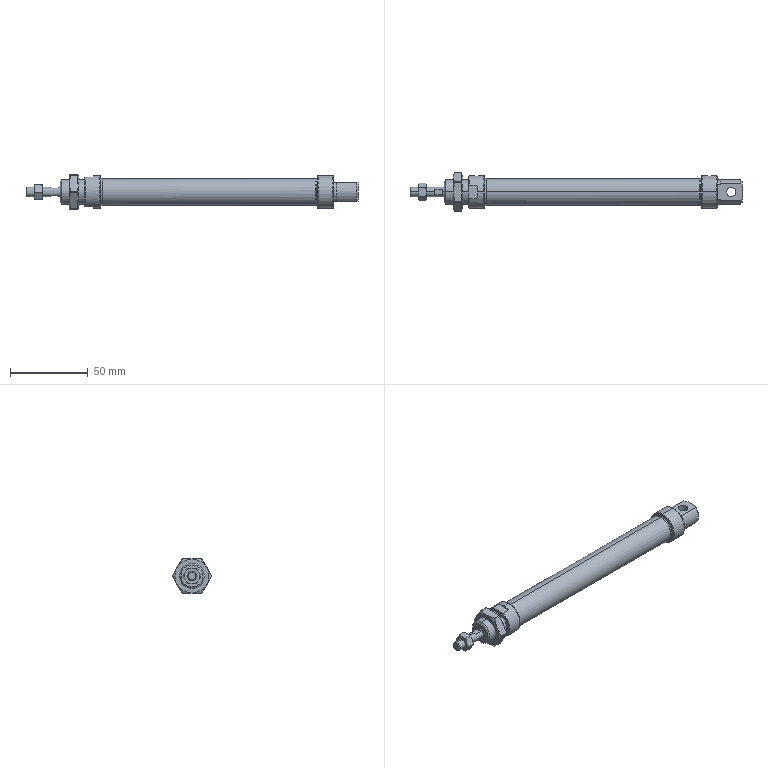Part | SolidWorks | features BaseBody 4, MoveFace 2 | 4 solids | 137 faces | box 214 x 25 x 22 mm | volume 42451 mm3 | plane 46 | cylinder 42 | cone 41 | spline 8 | commonest cylinder face diameters 6 x6 16 x6 17.4 x6 25 x6 4.134 x4 21 x4